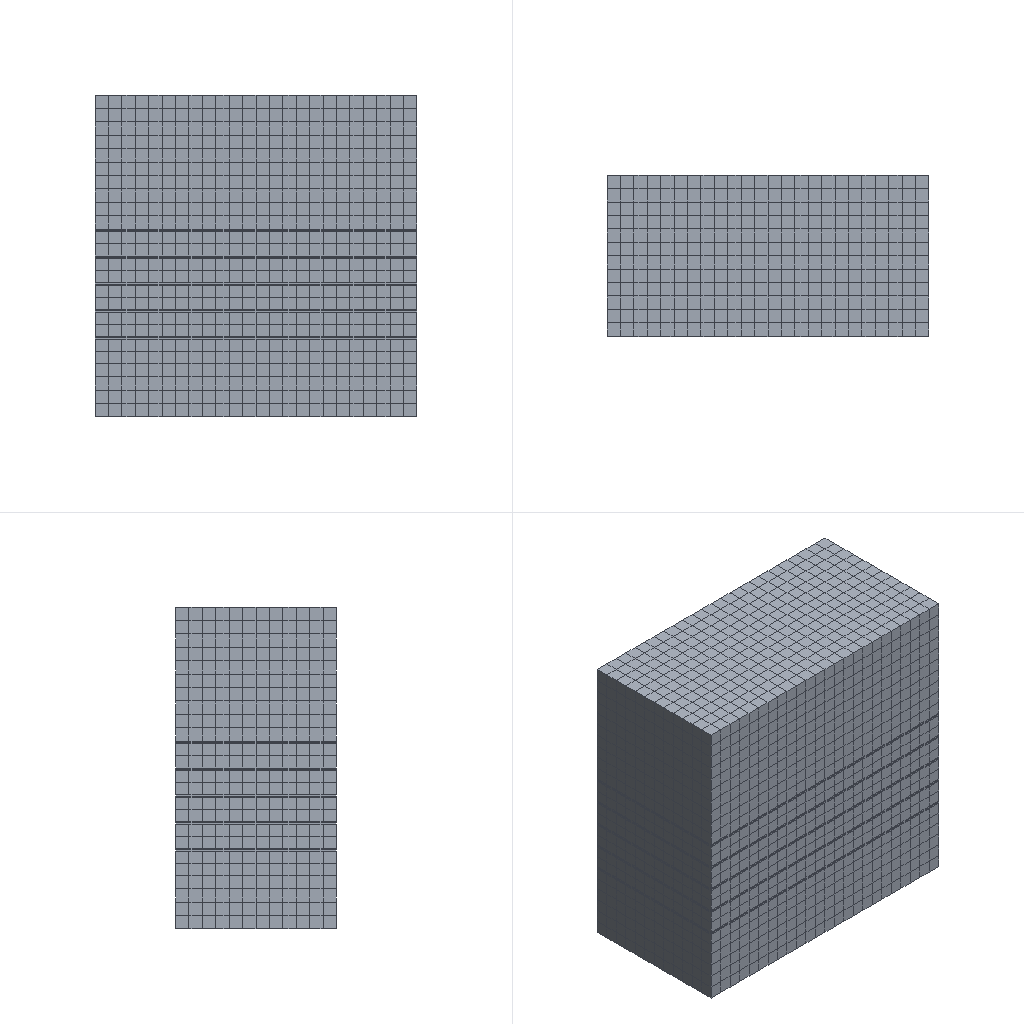Simulation study | abaqus
Set-up summary:
category,name,step,type,value,unit,region
solver,abaqus
solver,version,,,Abaqus/Standard 2020
units,not stated in the deck,,not stated
analysis,deck,,transient,transient
load_step,Step-1,Step-1,transient
load_step,Step-2,Step-2,transient
load_step,requested,,,2
mesh,nodes,,,11845
mesh,elements,,,10259
element_type,C3D8,,solid,9792
element_type,R3D4,,rigid,467
load,load commands in deck,,count,1
bc,support commands in deck,,count,13
material,CR,,in results
material,CRN,,in results
material,DLC,,in results
material,YG6,,in results
check,setup vs results,,match,"per instance, exact: element labels, types and connectivity; labels of the nodes the elements use; coordinates of those nodes at SINGLE_PRECISION in 2 of 2 instance(s)"
Abaqus input file, long lists of numbers shortened:
*Heading
** Job name: Job-2 Model name: Model-1
** Generated by: Abaqus/CAE 2020
*Preprint, echo=NO, model=NO, history=NO, contact=NO
**
** PARTS
**
*Part, name=work
*Node
      1, 0.0012,           0., 0.0002
      2, 0.0012, -0.0006, 0.0002
** (11373 more lines like these left out)
*Element, type=C3D8
   1,  154, 1229, 5810, 1091,    1,   53, 1025,   80
   2, 1229, 1230, 5811, 5810,   53,   54, 1026, 1025
** (9790 more lines like these left out)
*Nset, nset=Set-1
    45,    46,    47,    48,    49,    50,    51,    52,   850,   851,   852,   853,   854,   855,   856,   857
   858,   859,   860,   863,   864,   865,   866,   867,   868,   869,   870,   871,   872,   873,   875,   876
** (222 more lines like these left out)
*Elset, elset=Set-1, generate
 6913,  9792,     1
*Nset, nset=Set-2
   41,   42,   43,   44,   45,   46,   47,   48,  778,  779,  780,  781,  782,  783,  784,  785
  786,  787,  788,  791,  792,  793,  794,  795,  796,  797,  798,  799,  800,  801,  803,  804
** (59 more lines like these left out)
*Elset, elset=Set-2, generate
 6337,  6912,     1
*Nset, nset=Set-3
   33,   34,   35,   36,   37,   38,   39,   40,  634,  635,  636,  637,  638,  639,  640,  641
  642,  643,  644,  647,  648,  649,  650,  651,  652,  653,  654,  655,  656,  657,  659,  660
** (59 more lines like these left out)
*Elset, elset=Set-3, generate
 5185,  5760,     1
*Nset, nset=Set-4
   25,   26,   27,   28,   29,   30,   31,   32,  490,  491,  492,  493,  494,  495,  496,  497
  498,  499,  500,  503,  504,  505,  506,  507,  508,  509,  510,  511,  512,  513,  515,  516
** (59 more lines like these left out)
*Elset, elset=Set-4, generate
 4033,  4608,     1
*Nset, nset=Set-5
   37,   38,   39,   40,   41,   42,   43,   44,  705,  706,  707,  708,  709,  710,  711,  712
  713,  714,  715,  718,  719,  720,  721,  722,  723,  724,  725,  726,  727,  728,  731,  732
** (59 more lines like these left out)
*Elset, elset=Set-5, generate
 5761,  6336,     1
*Nset, nset=Set-6
   21,   22,   23,   24,   25,   26,   27,   28,   29,   30,   31,   32,   33,   34,   35,   36
  417,  418,  419,  420,  421,  422,  423,  424,  425,  426,  427,  430,  431,  432,  433,  434
** (120 more lines like these left out)
*Elset, elset=Set-6
 3457, 3458, 3459, 3460, 3461, 3462, 3463, 3464, 3465, 3466, 3467, 3468, 3469, 3470, 3471, 3472
 3473, 3474, 3475, 3476, 3477, 3478, 3479, 3480, 3481, 3482, 3483, 3484, 3485, 3486, 3487, 3488
** (70 more lines like these left out)
*Nset, nset=Set-9
    9,   10,   11,   12,   13,   14,   15,   16,   17,   18,   19,   20,   21,   22,   23,   24
  202,  203,  204,  205,  206,  207,  208,  209,  210,  211,  212,  215,  216,  217,  218,  219
** (120 more lines like these left out)
*Elset, elset=Set-9
 1729, 1730, 1731, 1732, 1733, 1734, 1735, 1736, 1737, 1738, 1739, 1740, 1741, 1742, 1743, 1744
 1745, 1746, 1747, 1748, 1749, 1750, 1751, 1752, 1753, 1754, 1755, 1756, 1757, 1758, 1759, 1760
** (70 more lines like these left out)
*Nset, nset=Set-10
    1,    2,    5,    8,    9,   10,   11,   12,   13,   14,   15,   16,   17,   18,   19,   20
   53,   54,   55,   56,   57,   58,   59,   60,   61,   62,   63,   81,   82,   83,   84,   85
** (120 more lines like these left out)
*Elset, elset=Set-10
 1153, 1154, 1155, 1156, 1157, 1158, 1159, 1160, 1161, 1162, 1163, 1164, 1165, 1166, 1167, 1168
 1169, 1170, 1171, 1172, 1173, 1174, 1175, 1176, 1177, 1178, 1179, 1180, 1181, 1182, 1183, 1184
** (70 more lines like these left out)
*Nset, nset=Set-11
    1,    2,    3,    4,    5,    6,    7,    8,   53,   54,   55,   56,   57,   58,   59,   60
   61,   62,   63,   64,   65,   66,   67,   68,   69,   70,   71,   72,   73,   74,   75,   76
** (100 more lines like these left out)
*Elset, elset=Set-11, generate
    1,  1152,     1
** Section: yg6
*Solid Section, elset=Set-11, material=yg6
,
** Section: crN
*Solid Section, elset=Set-10, material=crN
,
** Section: cr
*Solid Section, elset=Set-9, material=cr
,
** Section: crN
*Solid Section, elset=Set-6, material=crN
,
** Section: cr
*Solid Section, elset=Set-4, material=cr
,
** Section: cr
*Solid Section, elset=Set-3, material=cr
,
** Section: crN
*Solid Section, elset=Set-5, material=crN
,
** Section: cr
*Solid Section, elset=Set-2, material=cr
,
** Section: dlc
*Solid Section, elset=Set-1, material=DLC
,
*End Part
**
*Part, name=zhui
*Node
      1, 0.0003, -0.0005196,           0.
      2,           0.,           0.,           0.
** (467 more lines like these left out)
*Element, type=R3D4
 1, 120,  95,  40,  41
 2,  39,  40,  95,  97
** (465 more lines like these left out)
*Node
    470, 5.29395592e-20, -0.0003464, 9.20947787e-05
*Nset, nset=zhui-RefPt_, internal
470,
*Elset, elset=zhui, generate
   1,  467,    1
*End Part
**
**
** ASSEMBLY
**
*Assembly, name=Assembly
**
*Instance, name=work-1, part=work
*End Instance
**
*Instance, name=zhui-1, part=zhui
      0.0006, -5.39999999999999e-05,     0.001292
      0.0006, -5.39999999999999e-05,     0.001292,       0.0006,     0.9999,     0.001292,         180.
*End Instance
**
*Nset, nset=Set-1, instance=work-1
    3,    4,    6,    7,   67,   68,   69,   70,   71,   72,   73,   74,   75,   76,   77,   95
   96,   97,   98,   99,  100,  101,  102,  103,  104,  105,  109,  110,  111,  112,  113,  114
** (19 more lines like these left out)
*Elset, elset=Set-1, instance=work-1
   37,   38,   39,   40,   41,   42,   43,   44,   45,   46,   47,   48,   85,   86,   87,   88
   89,   90,   91,   92,   93,   94,   95,   96,  133,  134,  135,  136,  137,  138,  139,  140
** (16 more lines like these left out)
*Nset, nset=Set-2, instance=zhui-1
 470,
*Nset, nset=Set-3, instance=zhui-1
 470,
*Elset, elset=_m_Surf-1_SPOS, internal, instance=zhui-1, generate
   1,  248,    1
*Surface, type=ELEMENT, name=m_Surf-1
_m_Surf-1_SPOS, SPOS
*Elset, elset=_s_Surf-1_S5, internal, instance=work-1
 7021, 7022, 7023, 7024, 7025, 7026, 7027, 7028, 7029, 7030, 7031, 7032, 7141, 7142, 7143, 7144
 7145, 7146, 7147, 7148, 7149, 7150, 7151, 7152, 7261, 7262, 7263, 7264, 7265, 7266, 7267, 7268
** (16 more lines like these left out)
*Surface, type=ELEMENT, name=s_Surf-1
_s_Surf-1_S5, S5
*Rigid Body, ref node=zhui-1.zhui-RefPt_, elset=zhui-1.zhui
*End Assembly
**
** MATERIALS
**
*Material, name=DLC
*Density
 4e-09,
*Elastic
258800., 0.3
*Material, name=cr
*Density
 7.19e-09,
*Elastic
275000., 0.21
*Plastic
2000.,  0.
5000., 0.1
5500.,  1.
*Material, name=crN
*Density
 5.9e-09,
*Elastic
490000., 0.21
*Plastic
10000.,   0.
15000., 0.01
25000., 0.05
*Material, name=yg6
*Density
 1.5e-08,
*Elastic
71000., 0.3
*Plastic
3000.,0.
**
** INTERACTION PROPERTIES
**
*Surface Interaction, name=IntProp-1
1.,
*Friction, slip tolerance=0.005
 0.3,
*Surface Behavior, pressure-overclosure=HARD
**
** BOUNDARY CONDITIONS
**
** Name: BC-1 Type: 对称/反对称/完全固定
*Boundary
Set-1, ENCASTRE
**
** INTERACTIONS
**
** Interaction: Int-1
*Contact Pair, interaction=IntProp-1, type=SURFACE TO SURFACE
s_Surf-1, m_Surf-1
** Interaction: Int-2
*Contact
*Contact Inclusions, ALL EXTERIOR
*Contact Property Assignment
 ,  , IntProp-1
** ----------------------------------------------------------------
**
** STEP: Step-1
**
*Step, name=Step-1, nlgeom=YES, inc=10000
*Dynamic
0.001,10.,0.0001
**
** BOUNDARY CONDITIONS
**
** Name: BC-2 Type: 位移/转角
*Boundary
Set-2, 1, 1
Set-2, 2, 2
Set-2, 3, 3, -5e-05
Set-2, 4, 4
Set-2, 5, 5
Set-2, 6, 6
**
** OUTPUT REQUESTS
**
*Restart, write, frequency=0
**
** FIELD OUTPUT: F-Output-1
**
*Output, field, frequency=1
*Node Output
A, CF, RF, U, V
*Element Output, directions=YES
E, LE, MISES, PE, PEEQ, PEMAG, S
*Contact Output
CDISP, CSTRESS
**
** HISTORY OUTPUT: H-Output-1
**
*Output, history, variable=PRESELECT
*End Step
** ----------------------------------------------------------------
**
** STEP: Step-2
**
*Step, name=Step-2, nlgeom=YES, inc=1000
*Dynamic
0.01,1.,1e-05
**
** BOUNDARY CONDITIONS
**
** Name: BC-1 Type: 对称/反对称/完全固定
*Boundary, op=NEW
Set-1, ENCASTRE
** Name: BC-2 Type: 位移/转角
*Boundary, op=NEW
Set-2, 1, 1
Set-2, 2, 2
Set-2, 4, 4
Set-2, 5, 5
Set-2, 6, 6
**
** OUTPUT REQUESTS
**
*Restart, write, frequency=0
**
** FIELD OUTPUT: F-Output-1
**
*Output, field, frequency=1
*Node Output
A, CF, RF, U, V
*Element Output, directions=YES
E, LE, MISES, PE, PEEQ, PEMAG, S
*Contact Output
CDISP, CSTRESS
**
** HISTORY OUTPUT: H-Output-1
**
*Output, history, variable=PRESELECT
*End Step
Results summary:
result,step,,completed,increments=31 time=10.0/10.0
result,step,,partial,increments=6 time=0.02534/1.0
result,analysis,,,transient
result,last_loadstep,,,2
result,primary field,,,U
result,reaction total,,FX,-0.0,model units
result,reaction total,,FY,-0.000184,model units
result,reaction total,,FZ,0.000801,model units